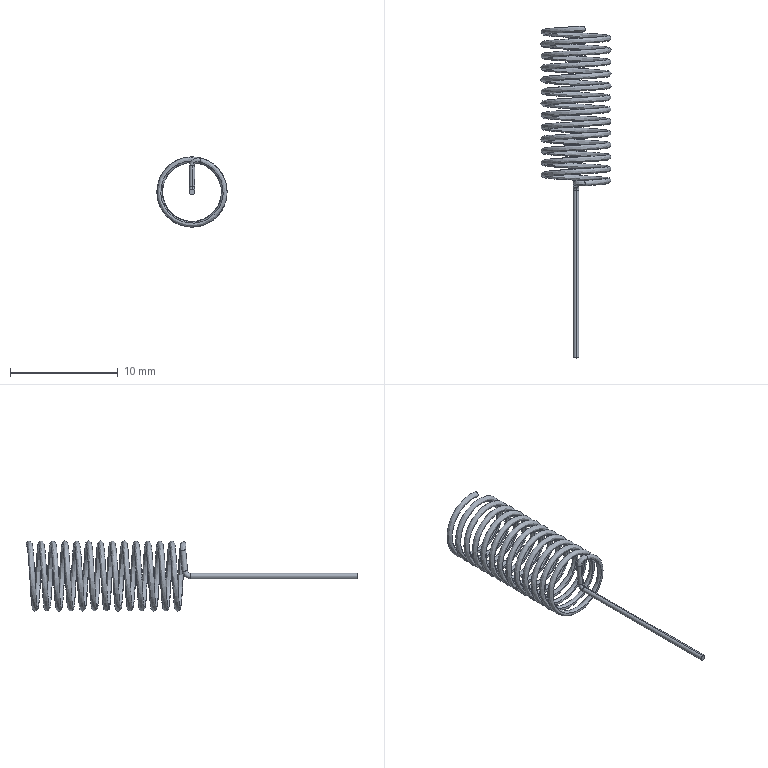Part | SolidWorks | features 3DProfileFeature 2, Helix 1, Sweep 1 | 1 solid | 12 faces | box 6.5 x 30.75 x 6.5 mm | volume 51.975 mm3 | spline 4 | cylinder 4 | torus 2 | plane 2 | commonest cylinder face diameters 0.5 x4